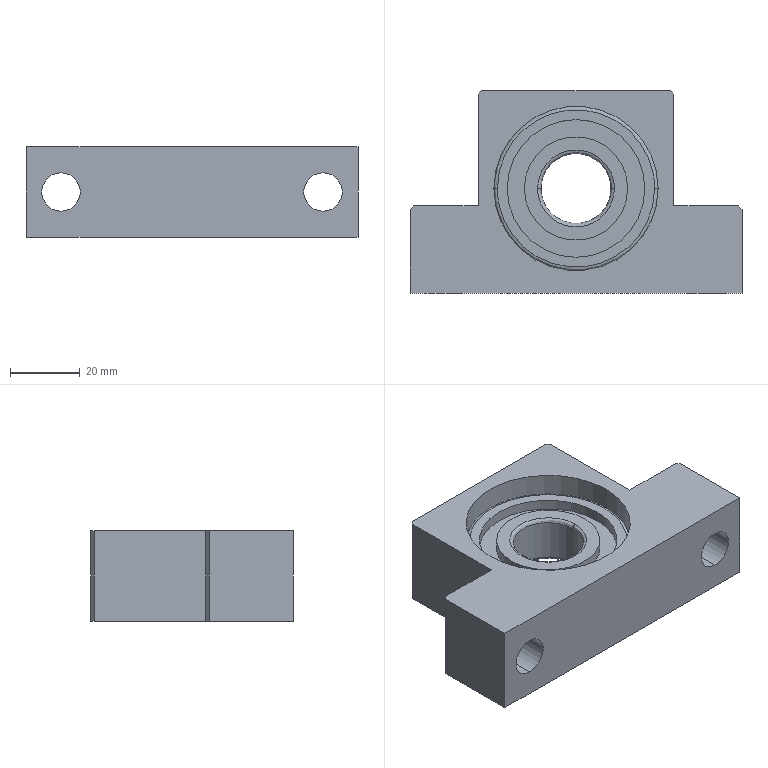Part | STEP file | LEB31-20 | 1 solid | 46 faces | box 95 x 58 x 26 mm | volume 76469 mm3 | plane 20 | cylinder 18 | spline 8 | commonest cylinder face diameters 11 x4 29.6 x4 39.4 x4 47 x4 20 x2